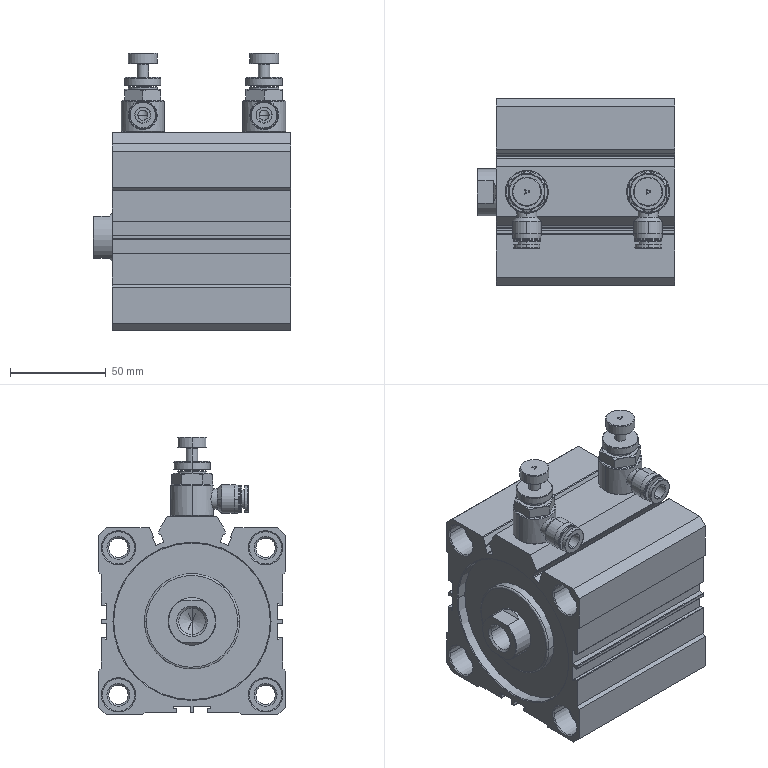Part | SolidWorks | features BaseBody 4 | 4 solids | 485 faces | box 103.5 x 98 x 145.5 mm | volume 625732 mm3 | plane 183 | cylinder 172 | cone 114 | spline 16 | commonest cylinder face diameters 0.4 x35 17 x16 0.8 x15 6 x8 10.106 x8 14.4 x8